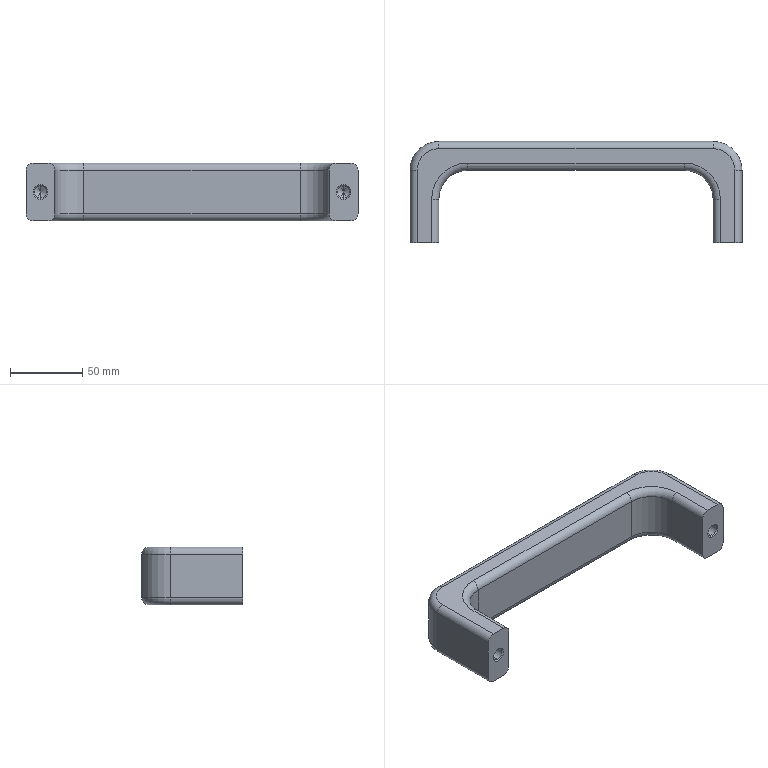Part | SolidWorks | features Fillet 2, 3DProfileFeature 1, Extrusion 1, HoleWzd 1 | 1 solid | 46 faces | box 230 x 70 x 40 mm | volume 254336 mm3 | cylinder 20 | plane 10 | cone 8 | torus 8 | commonest cylinder face diameters 10 x12 8.5 x4 40 x4
STEP:
#1=CARTESIAN_POINT('',(-31.,226.775,4.25));
#2=VERTEX_POINT('',#1);
#3=CARTESIAN_POINT('',(-31.,226.775,-4.25));
#4=VERTEX_POINT('',#3);
#5=CARTESIAN_POINT('',(-31.,226.775,0.));
#6=DIRECTION('',(0.,-1.,0.));
#7=DIRECTION('',(0.,0.,-1.));
#8=AXIS2_PLACEMENT_3D('',#5,#6,#7);
#9=CIRCLE('',#8,4.25);
#10=EDGE_CURVE('',#2,#4,#9,.T.);
#11=ORIENTED_EDGE('',*,*,#10,.F.);
#12=CARTESIAN_POINT('',(-31.,226.,5.025));
#13=VERTEX_POINT('',#12);
#14=CARTESIAN_POINT('',(-31.,226.,5.025));
#15=DIRECTION('',(0.,-0.7071,0.7071));
#16=VECTOR('',#15,1000.);
#17=LINE('',#14,#16);
#18=EDGE_CURVE('',#2,#13,#17,.T.);
#19=ORIENTED_EDGE('',*,*,#18,.T.);
#20=CARTESIAN_POINT('',(-31.,226.,-5.025));
#21=VERTEX_POINT('',#20);
#22=CARTESIAN_POINT('',(-31.,226.,0.));
#23=DIRECTION('',(0.,-1.,0.));
#24=DIRECTION('',(0.,0.,-1.));
#25=AXIS2_PLACEMENT_3D('',#22,#23,#24);
#26=CIRCLE('',#25,5.025);
#27=EDGE_CURVE('',#13,#21,#26,.T.);
#28=ORIENTED_EDGE('',*,*,#27,.T.);
#29=CARTESIAN_POINT('',(-31.,226.,-5.025));
#30=DIRECTION('',(0.,-0.7071,-0.7071));
#31=VECTOR('',#30,1000.);
#32=LINE('',#29,#31);
#33=EDGE_CURVE('',#4,#21,#32,.T.);
#34=ORIENTED_EDGE('',*,*,#33,.F.);
#35=EDGE_LOOP('',(#11,#19,#28,#34));
#36=FACE_OUTER_BOUND('',#35,.T.);
#37=CARTESIAN_POINT('',(-31.,226.,0.));
#38=DIRECTION('',(0.,-1.,0.));
#39=DIRECTION('',(0.,0.,-1.));
#40=AXIS2_PLACEMENT_3D('',#37,#38,#39);
#41=CONICAL_SURFACE('',#40,5.025,0.7854);
#42=ADVANCED_FACE('',(#36),#41,.F.);
#43=CARTESIAN_POINT('',(-31.,251.,4.25));
#44=VERTEX_POINT('',#43);
#45=CARTESIAN_POINT('',(-31.,251.,-4.25));
#46=VERTEX_POINT('',#45);
#47=CARTESIAN_POINT('',(-31.,251.,0.));
#48=DIRECTION('',(0.,-1.,0.));
#49=DIRECTION('',(0.,0.,-1.));
#50=AXIS2_PLACEMENT_3D('',#47,#48,#49);
#51=CIRCLE('',#50,4.25);
#52=EDGE_CURVE('',#44,#46,#51,.T.);
#53=ORIENTED_EDGE('',*,*,#52,.F.);
#54=CARTESIAN_POINT('',(-31.,226.,4.25));
#55=DIRECTION('',(0.,-1.,0.));
#56=VECTOR('',#55,1000.);
#57=LINE('',#54,#56);
#58=EDGE_CURVE('',#44,#2,#57,.T.);
#59=ORIENTED_EDGE('',*,*,#58,.T.);
#60=ORIENTED_EDGE('',*,*,#10,.T.);
#61=CARTESIAN_POINT('',(-31.,226.,-4.25));
#62=DIRECTION('',(0.,-1.,0.));
#63=VECTOR('',#62,1000.);
#64=LINE('',#61,#63);
#65=EDGE_CURVE('',#46,#4,#64,.T.);
#66=ORIENTED_EDGE('',*,*,#65,.F.);
#67=EDGE_LOOP('',(#53,#59,#60,#66));
#68=FACE_OUTER_BOUND('',#67,.T.);
#69=CARTESIAN_POINT('',(-31.,226.,0.));
#70=DIRECTION('',(0.,-1.,0.));
#71=DIRECTION('',(0.,0.,-1.));
#72=AXIS2_PLACEMENT_3D('',#69,#70,#71);
#73=CYLINDRICAL_SURFACE('',#72,4.25);
#74=ADVANCED_FACE('',(#68),#73,.F.);
#75=CARTESIAN_POINT('',(-31.,253.554,0.));
#76=VERTEX_POINT('',#75);
#77=CARTESIAN_POINT('',(-31.,251.,-4.25));
#78=DIRECTION('',(0.,-0.515,-0.8572));
#79=VECTOR('',#78,1000.);
#80=LINE('',#77,#79);
#81=EDGE_CURVE('',#76,#46,#80,.T.);
#82=ORIENTED_EDGE('',*,*,#81,.F.);
#83=CARTESIAN_POINT('',(-31.,251.,4.25));
#84=DIRECTION('',(0.,-0.515,0.8572));
#85=VECTOR('',#84,1000.);
#86=LINE('',#83,#85);
#87=EDGE_CURVE('',#76,#44,#86,.T.);
#88=ORIENTED_EDGE('',*,*,#87,.T.);
#89=ORIENTED_EDGE('',*,*,#52,.T.);
#90=EDGE_LOOP('',(#82,#88,#89));
#91=FACE_OUTER_BOUND('',#90,.T.);
#92=CARTESIAN_POINT('',(-31.,251.,0.));
#93=DIRECTION('',(0.,-1.,0.));
#94=DIRECTION('',(0.,0.,-1.));
#95=AXIS2_PLACEMENT_3D('',#92,#93,#94);
#96=CONICAL_SURFACE('',#95,4.25,1.03);
#97=ADVANCED_FACE('',(#91),#96,.F.);
#98=CARTESIAN_POINT('',(179.,226.775,4.25));
#99=VERTEX_POINT('',#98);
#100=CARTESIAN_POINT('',(179.,226.775,-4.25));
#101=VERTEX_POINT('',#100);
#102=CARTESIAN_POINT('',(179.,226.775,0.));
#103=DIRECTION('',(0.,-1.,0.));
#104=DIRECTION('',(0.,0.,-1.));
#105=AXIS2_PLACEMENT_3D('',#102,#103,#104);
#106=CIRCLE('',#105,4.25);
#107=EDGE_CURVE('',#99,#101,#106,.T.);
#108=ORIENTED_EDGE('',*,*,#107,.F.);
#109=CARTESIAN_POINT('',(179.,226.,5.025));
#110=VERTEX_POINT('',#109);
#111=CARTESIAN_POINT('',(179.,226.,5.025));
#112=DIRECTION('',(0.,-0.7071,0.7071));
#113=VECTOR('',#112,1000.);
#114=LINE('',#111,#113);
#115=EDGE_CURVE('',#99,#110,#114,.T.);
#116=ORIENTED_EDGE('',*,*,#115,.T.);
#117=CARTESIAN_POINT('',(179.,226.,-5.025));
#118=VERTEX_POINT('',#117);
#119=CARTESIAN_POINT('',(179.,226.,0.));
#120=DIRECTION('',(0.,-1.,0.));
#121=DIRECTION('',(0.,0.,-1.));
#122=AXIS2_PLACEMENT_3D('',#119,#120,#121);
#123=CIRCLE('',#122,5.025);
#124=EDGE_CURVE('',#110,#118,#123,.T.);
#125=ORIENTED_EDGE('',*,*,#124,.T.);
#126=CARTESIAN_POINT('',(179.,226.,-5.025));
#127=DIRECTION('',(0.,-0.7071,-0.7071));
#128=VECTOR('',#127,1000.);
#129=LINE('',#126,#128);
#130=EDGE_CURVE('',#101,#118,#129,.T.);
#131=ORIENTED_EDGE('',*,*,#130,.F.);
#132=EDGE_LOOP('',(#108,#116,#125,#131));
#133=FACE_OUTER_BOUND('',#132,.T.);
#134=CARTESIAN_POINT('',(179.,226.,0.));
#135=DIRECTION('',(0.,-1.,0.));
#136=DIRECTION('',(0.,0.,-1.));
#137=AXIS2_PLACEMENT_3D('',#134,#135,#136);
#138=CONICAL_SURFACE('',#137,5.025,0.7854);
#139=ADVANCED_FACE('',(#133),#138,.F.);
#140=CARTESIAN_POINT('',(179.,251.,4.25));
#141=VERTEX_POINT('',#140);
#142=CARTESIAN_POINT('',(179.,251.,-4.25));
#143=VERTEX_POINT('',#142);
#144=CARTESIAN_POINT('',(179.,251.,0.));
#145=DIRECTION('',(0.,-1.,0.));
#146=DIRECTION('',(0.,0.,-1.));
#147=AXIS2_PLACEMENT_3D('',#144,#145,#146);
#148=CIRCLE('',#147,4.25);
#149=EDGE_CURVE('',#141,#143,#148,.T.);
#150=ORIENTED_EDGE('',*,*,#149,.F.);
#151=CARTESIAN_POINT('',(179.,226.,4.25));
#152=DIRECTION('',(0.,-1.,0.));
#153=VECTOR('',#152,1000.);
#154=LINE('',#151,#153);
#155=EDGE_CURVE('',#141,#99,#154,.T.);
#156=ORIENTED_EDGE('',*,*,#155,.T.);
#157=ORIENTED_EDGE('',*,*,#107,.T.);
#158=CARTESIAN_POINT('',(179.,226.,-4.25));
#159=DIRECTION('',(0.,-1.,0.));
#160=VECTOR('',#159,1000.);
#161=LINE('',#158,#160);
#162=EDGE_CURVE('',#143,#101,#161,.T.);
#163=ORIENTED_EDGE('',*,*,#162,.F.);
#164=EDGE_LOOP('',(#150,#156,#157,#163));
#165=FACE_OUTER_BOUND('',#164,.T.);
#166=CARTESIAN_POINT('',(179.,226.,0.));
#167=DIRECTION('',(0.,-1.,0.));
#168=DIRECTION('',(0.,0.,-1.));
#169=AXIS2_PLACEMENT_3D('',#166,#167,#168);
#170=CYLINDRICAL_SURFACE('',#169,4.25);
#171=ADVANCED_FACE('',(#165),#170,.F.);
#172=CARTESIAN_POINT('',(179.,253.554,0.));
#173=VERTEX_POINT('',#172);
#174=CARTESIAN_POINT('',(179.,251.,-4.25));
#175=DIRECTION('',(0.,-0.515,-0.8572));
#176=VECTOR('',#175,1000.);
#177=LINE('',#174,#176);
#178=EDGE_CURVE('',#173,#143,#177,.T.);
#179=ORIENTED_EDGE('',*,*,#178,.F.);
#180=CARTESIAN_POINT('',(179.,251.,4.25));
#181=DIRECTION('',(0.,-0.515,0.8572));
#182=VECTOR('',#181,1000.);
#183=LINE('',#180,#182);
#184=EDGE_CURVE('',#173,#141,#183,.T.);
#185=ORIENTED_EDGE('',*,*,#184,.T.);
#186=ORIENTED_EDGE('',*,*,#149,.T.);
#187=EDGE_LOOP('',(#179,#185,#186));
#188=FACE_OUTER_BOUND('',#187,.T.);
#189=CARTESIAN_POINT('',(179.,251.,0.));
#190=DIRECTION('',(0.,-1.,0.));
#191=DIRECTION('',(0.,0.,-1.));
#192=AXIS2_PLACEMENT_3D('',#189,#190,#191);
#193=CONICAL_SURFACE('',#192,4.25,1.03);
#194=ADVANCED_FACE('',(#188),#193,.F.);
#195=CARTESIAN_POINT('',(-31.,226.,0.));
#196=DIRECTION('',(0.,-1.,0.));
#197=DIRECTION('',(0.,0.,-1.));
#198=AXIS2_PLACEMENT_3D('',#195,#196,#197);
#199=CIRCLE('',#198,5.025);
#200=EDGE_CURVE('',#21,#13,#199,.T.);
#201=ORIENTED_EDGE('',*,*,#200,.F.);
#202=ORIENTED_EDGE('',*,*,#27,.F.);
#203=EDGE_LOOP('',(#201,#202));
#204=FACE_BOUND('',#203,.T.);
#205=CARTESIAN_POINT('',(-41.,226.,15.));
#206=VERTEX_POINT('',#205);
#207=CARTESIAN_POINT('',(-41.,226.,-15.));
#208=VERTEX_POINT('',#207);
#209=CARTESIAN_POINT('',(-41.,226.,20.));
#210=DIRECTION('',(0.,0.,-1.));
#211=VECTOR('',#210,1000.);
#212=LINE('',#209,#211);
#213=EDGE_CURVE('',#206,#208,#212,.T.);
#214=ORIENTED_EDGE('',*,*,#213,.T.);
#215=CARTESIAN_POINT('',(-36.,226.,-20.));
#216=VERTEX_POINT('',#215);
#217=CARTESIAN_POINT('',(-36.,226.,-15.));
#218=DIRECTION('',(0.,-1.,0.));
#219=DIRECTION('',(0.,0.,-1.));
#220=AXIS2_PLACEMENT_3D('',#217,#218,#219);
#221=CIRCLE('',#220,5.);
#222=EDGE_CURVE('',#208,#216,#221,.T.);
#223=ORIENTED_EDGE('',*,*,#222,.T.);
#224=CARTESIAN_POINT('',(-26.,226.,-20.));
#225=VERTEX_POINT('',#224);
#226=CARTESIAN_POINT('',(-21.,226.,-20.));
#227=DIRECTION('',(-1.,0.,0.));
#228=VECTOR('',#227,1000.);
#229=LINE('',#226,#228);
#230=EDGE_CURVE('',#225,#216,#229,.T.);
#231=ORIENTED_EDGE('',*,*,#230,.F.);
#232=CARTESIAN_POINT('',(-21.,226.,-15.));
#233=VERTEX_POINT('',#232);
#234=CARTESIAN_POINT('',(-26.,226.,-15.));
#235=DIRECTION('',(0.,-1.,0.));
#236=DIRECTION('',(0.,0.,-1.));
#237=AXIS2_PLACEMENT_3D('',#234,#235,#236);
#238=CIRCLE('',#237,5.);
#239=EDGE_CURVE('',#225,#233,#238,.T.);
#240=ORIENTED_EDGE('',*,*,#239,.T.);
#241=CARTESIAN_POINT('',(-21.,226.,15.));
#242=VERTEX_POINT('',#241);
#243=CARTESIAN_POINT('',(-21.,226.,20.));
#244=DIRECTION('',(0.,0.,-1.));
#245=VECTOR('',#244,1000.);
#246=LINE('',#243,#245);
#247=EDGE_CURVE('',#242,#233,#246,.T.);
#248=ORIENTED_EDGE('',*,*,#247,.F.);
#249=CARTESIAN_POINT('',(-26.,226.,20.));
#250=VERTEX_POINT('',#249);
#251=CARTESIAN_POINT('',(-26.,226.,15.));
#252=DIRECTION('',(0.,-1.,0.));
#253=DIRECTION('',(0.,0.,-1.));
#254=AXIS2_PLACEMENT_3D('',#251,#252,#253);
#255=CIRCLE('',#254,5.);
#256=EDGE_CURVE('',#242,#250,#255,.T.);
#257=ORIENTED_EDGE('',*,*,#256,.T.);
#258=CARTESIAN_POINT('',(-36.,226.,20.));
#259=VERTEX_POINT('',#258);
#260=CARTESIAN_POINT('',(-21.,226.,20.));
#261=DIRECTION('',(-1.,0.,0.));
#262=VECTOR('',#261,1000.);
#263=LINE('',#260,#262);
#264=EDGE_CURVE('',#250,#259,#263,.T.);
#265=ORIENTED_EDGE('',*,*,#264,.T.);
#266=CARTESIAN_POINT('',(-36.,226.,15.));
#267=DIRECTION('',(0.,-1.,0.));
#268=DIRECTION('',(0.,0.,-1.));
#269=AXIS2_PLACEMENT_3D('',#266,#267,#268);
#270=CIRCLE('',#269,5.);
#271=EDGE_CURVE('',#259,#206,#270,.T.);
#272=ORIENTED_EDGE('',*,*,#271,.T.);
#273=EDGE_LOOP('',(#214,#223,#231,#240,#248,#257,#265,#272));
#274=FACE_OUTER_BOUND('',#273,.T.);
#275=CARTESIAN_POINT('',(-21.,226.,20.));
#276=DIRECTION('',(0.,-1.,0.));
#277=DIRECTION('',(0.,0.,-1.));
#278=AXIS2_PLACEMENT_3D('',#275,#276,#277);
#279=PLANE('',#278);
#280=ADVANCED_FACE('',(#204,#274),#279,.T.);
#281=ORIENTED_EDGE('',*,*,#247,.T.);
#282=CARTESIAN_POINT('',(-21.,256.,-15.));
#283=VERTEX_POINT('',#282);
#284=CARTESIAN_POINT('',(-21.,256.,-15.));
#285=DIRECTION('',(0.,1.,0.));
#286=VECTOR('',#285,1000.);
#287=LINE('',#284,#286);
#288=EDGE_CURVE('',#233,#283,#287,.T.);
#289=ORIENTED_EDGE('',*,*,#288,.T.);
#290=CARTESIAN_POINT('',(-21.,256.,15.));
#291=VERTEX_POINT('',#290);
#292=CARTESIAN_POINT('',(-21.,256.,20.));
#293=DIRECTION('',(0.,0.,1.));
#294=VECTOR('',#293,1000.);
#295=LINE('',#292,#294);
#296=EDGE_CURVE('',#283,#291,#295,.T.);
#297=ORIENTED_EDGE('',*,*,#296,.T.);
#298=CARTESIAN_POINT('',(-21.,226.,15.));
#299=DIRECTION('',(0.,-1.,0.));
#300=VECTOR('',#299,1000.);
#301=LINE('',#298,#300);
#302=EDGE_CURVE('',#291,#242,#301,.T.);
#303=ORIENTED_EDGE('',*,*,#302,.T.);
#304=EDGE_LOOP('',(#281,#289,#297,#303));
#305=FACE_OUTER_BOUND('',#304,.T.);
#306=CARTESIAN_POINT('',(-21.,226.,20.));
#307=DIRECTION('',(-1.,0.,0.));
#308=DIRECTION('',(0.,0.,1.));
#309=AXIS2_PLACEMENT_3D('',#306,#307,#308);
#310=PLANE('',#309);
#311=ADVANCED_FACE('',(#305),#310,.F.);
#312=CARTESIAN_POINT('',(-1.,276.,15.));
#313=VERTEX_POINT('',#312);
#314=CARTESIAN_POINT('',(-1.,276.,-15.));
#315=VERTEX_POINT('',#314);
#316=CARTESIAN_POINT('',(-1.,276.,-20.));
#317=DIRECTION('',(0.,0.,-1.));
#318=VECTOR('',#317,1000.);
#319=LINE('',#316,#318);
#320=EDGE_CURVE('',#313,#315,#319,.T.);
#321=ORIENTED_EDGE('',*,*,#320,.T.);
#322=CARTESIAN_POINT('',(149.,276.,-15.));
#323=VERTEX_POINT('',#322);
#324=CARTESIAN_POINT('',(149.,276.,-15.));
#325=DIRECTION('',(1.,0.,0.));
#326=VECTOR('',#325,1000.);
#327=LINE('',#324,#326);
#328=EDGE_CURVE('',#315,#323,#327,.T.);
#329=ORIENTED_EDGE('',*,*,#328,.T.);
#330=CARTESIAN_POINT('',(149.,276.,15.));
#331=VERTEX_POINT('',#330);
#332=CARTESIAN_POINT('',(149.,276.,20.));
#333=DIRECTION('',(0.,0.,1.));
#334=VECTOR('',#333,1000.);
#335=LINE('',#332,#334);
#336=EDGE_CURVE('',#323,#331,#335,.T.);
#337=ORIENTED_EDGE('',*,*,#336,.T.);
#338=CARTESIAN_POINT('',(-21.,276.,15.));
#339=DIRECTION('',(-1.,0.,0.));
#340=VECTOR('',#339,1000.);
#341=LINE('',#338,#340);
#342=EDGE_CURVE('',#331,#313,#341,.T.);
#343=ORIENTED_EDGE('',*,*,#342,.T.);
#344=EDGE_LOOP('',(#321,#329,#337,#343));
#345=FACE_OUTER_BOUND('',#344,.T.);
#346=CARTESIAN_POINT('',(-21.,276.,20.));
#347=DIRECTION('',(0.,1.,0.));
#348=DIRECTION('',(0.,0.,1.));
#349=AXIS2_PLACEMENT_3D('',#346,#347,#348);
#350=PLANE('',#349);
#351=ADVANCED_FACE('',(#345),#350,.F.);
#352=CARTESIAN_POINT('',(169.,256.,15.));
#353=VERTEX_POINT('',#352);
#354=CARTESIAN_POINT('',(169.,256.,-15.));
#355=VERTEX_POINT('',#354);
#356=CARTESIAN_POINT('',(169.,256.,-20.));
#357=DIRECTION('',(0.,0.,-1.));
#358=VECTOR('',#357,1000.);
#359=LINE('',#356,#358);
#360=EDGE_CURVE('',#353,#355,#359,.T.);
#361=ORIENTED_EDGE('',*,*,#360,.T.);
#362=CARTESIAN_POINT('',(169.,226.,-15.));
#363=VERTEX_POINT('',#362);
#364=CARTESIAN_POINT('',(169.,226.,-15.));
#365=DIRECTION('',(0.,-1.,0.));
#366=VECTOR('',#365,1000.);
#367=LINE('',#364,#366);
#368=EDGE_CURVE('',#355,#363,#367,.T.);
#369=ORIENTED_EDGE('',*,*,#368,.T.);
#370=CARTESIAN_POINT('',(169.,226.,15.));
#371=VERTEX_POINT('',#370);
#372=CARTESIAN_POINT('',(169.,226.,20.));
#373=DIRECTION('',(0.,0.,-1.));
#374=VECTOR('',#373,1000.);
#375=LINE('',#372,#374);
#376=EDGE_CURVE('',#371,#363,#375,.T.);
#377=ORIENTED_EDGE('',*,*,#376,.F.);
#378=CARTESIAN_POINT('',(169.,276.,15.));
#379=DIRECTION('',(0.,1.,0.));
#380=VECTOR('',#379,1000.);
#381=LINE('',#378,#380);
#382=EDGE_CURVE('',#371,#353,#381,.T.);
#383=ORIENTED_EDGE('',*,*,#382,.T.);
#384=EDGE_LOOP('',(#361,#369,#377,#383));
#385=FACE_OUTER_BOUND('',#384,.T.);
#386=CARTESIAN_POINT('',(169.,276.,20.));
#387=DIRECTION('',(1.,0.,0.));
#388=DIRECTION('',(0.,0.,-1.));
#389=AXIS2_PLACEMENT_3D('',#386,#387,#388);
#390=PLANE('',#389);
#391=ADVANCED_FACE('',(#385),#390,.F.);
#392=CARTESIAN_POINT('',(179.,226.,0.));
#393=DIRECTION('',(0.,-1.,0.));
#394=DIRECTION('',(0.,0.,-1.));
#395=AXIS2_PLACEMENT_3D('',#392,#393,#394);
#396=CIRCLE('',#395,5.025);
#397=EDGE_CURVE('',#118,#110,#396,.T.);
#398=ORIENTED_EDGE('',*,*,#397,.F.);
#399=ORIENTED_EDGE('',*,*,#124,.F.);
#400=EDGE_LOOP('',(#398,#399));
#401=FACE_BOUND('',#400,.T.);
#402=ORIENTED_EDGE('',*,*,#376,.T.);
#403=CARTESIAN_POINT('',(174.,226.,-20.));
#404=VERTEX_POINT('',#403);
#405=CARTESIAN_POINT('',(174.,226.,-15.));
#406=DIRECTION('',(0.,-1.,0.));
#407=DIRECTION('',(0.,0.,-1.));
#408=AXIS2_PLACEMENT_3D('',#405,#406,#407);
#409=CIRCLE('',#408,5.);
#410=EDGE_CURVE('',#363,#404,#409,.T.);
#411=ORIENTED_EDGE('',*,*,#410,.T.);
#412=CARTESIAN_POINT('',(184.,226.,-20.));
#413=VERTEX_POINT('',#412);
#414=CARTESIAN_POINT('',(189.,226.,-20.));
#415=DIRECTION('',(-1.,0.,0.));
#416=VECTOR('',#415,1000.);
#417=LINE('',#414,#416);
#418=EDGE_CURVE('',#413,#404,#417,.T.);
#419=ORIENTED_EDGE('',*,*,#418,.F.);
#420=CARTESIAN_POINT('',(189.,226.,-15.));
#421=VERTEX_POINT('',#420);
#422=CARTESIAN_POINT('',(184.,226.,-15.));
#423=DIRECTION('',(0.,-1.,0.));
#424=DIRECTION('',(0.,0.,-1.));
#425=AXIS2_PLACEMENT_3D('',#422,#423,#424);
#426=CIRCLE('',#425,5.);
#427=EDGE_CURVE('',#413,#421,#426,.T.);
#428=ORIENTED_EDGE('',*,*,#427,.T.);
#429=CARTESIAN_POINT('',(189.,226.,15.));
#430=VERTEX_POINT('',#429);
#431=CARTESIAN_POINT('',(189.,226.,20.));
#432=DIRECTION('',(0.,0.,-1.));
#433=VECTOR('',#432,1000.);
#434=LINE('',#431,#433);
#435=EDGE_CURVE('',#430,#421,#434,.T.);
#436=ORIENTED_EDGE('',*,*,#435,.F.);
#437=CARTESIAN_POINT('',(184.,226.,20.));
#438=VERTEX_POINT('',#437);
#439=CARTESIAN_POINT('',(184.,226.,15.));
#440=DIRECTION('',(0.,-1.,0.));
#441=DIRECTION('',(0.,0.,-1.));
#442=AXIS2_PLACEMENT_3D('',#439,#440,#441);
#443=CIRCLE('',#442,5.);
#444=EDGE_CURVE('',#430,#438,#443,.T.);
#445=ORIENTED_EDGE('',*,*,#444,.T.);
#446=CARTESIAN_POINT('',(174.,226.,20.));
#447=VERTEX_POINT('',#446);
#448=CARTESIAN_POINT('',(189.,226.,20.));
#449=DIRECTION('',(-1.,0.,0.));
#450=VECTOR('',#449,1000.);
#451=LINE('',#448,#450);
#452=EDGE_CURVE('',#438,#447,#451,.T.);
#453=ORIENTED_EDGE('',*,*,#452,.T.);
#454=CARTESIAN_POINT('',(174.,226.,15.));
#455=DIRECTION('',(0.,-1.,0.));
#456=DIRECTION('',(0.,0.,-1.));
#457=AXIS2_PLACEMENT_3D('',#454,#455,#456);
#458=CIRCLE('',#457,5.);
#459=EDGE_CURVE('',#447,#371,#458,.T.);
#460=ORIENTED_EDGE('',*,*,#459,.T.);
#461=EDGE_LOOP('',(#402,#411,#419,#428,#436,#445,#453,#460));
#462=FACE_OUTER_BOUND('',#461,.T.);
#463=CARTESIAN_POINT('',(189.,226.,20.));
#464=DIRECTION('',(0.,-1.,0.));
#465=DIRECTION('',(0.,0.,-1.));
#466=AXIS2_PLACEMENT_3D('',#463,#464,#465);
#467=PLANE('',#466);
#468=ADVANCED_FACE('',(#401,#462),#467,.T.);
#469=ORIENTED_EDGE('',*,*,#435,.T.);
#470=CARTESIAN_POINT('',(189.,276.,-15.));
#471=VERTEX_POINT('',#470);
#472=CARTESIAN_POINT('',(189.,296.,-15.));
#473=DIRECTION('',(0.,1.,0.));
#474=VECTOR('',#473,1000.);
#475=LINE('',#472,#474);
#476=EDGE_CURVE('',#421,#471,#475,.T.);
#477=ORIENTED_EDGE('',*,*,#476,.T.);
#478=CARTESIAN_POINT('',(189.,276.,15.));
#479=VERTEX_POINT('',#478);
#480=CARTESIAN_POINT('',(189.,276.,20.));
#481=DIRECTION('',(0.,0.,1.));
#482=VECTOR('',#481,1000.);
#483=LINE('',#480,#482);
#484=EDGE_CURVE('',#471,#479,#483,.T.);
#485=ORIENTED_EDGE('',*,*,#484,.T.);
#486=CARTESIAN_POINT('',(189.,226.,15.));
#487=DIRECTION('',(0.,-1.,0.));
#488=VECTOR('',#487,1000.);
#489=LINE('',#486,#488);
#490=EDGE_CURVE('',#479,#430,#489,.T.);
#491=ORIENTED_EDGE('',*,*,#490,.T.);
#492=EDGE_LOOP('',(#469,#477,#485,#491));
#493=FACE_OUTER_BOUND('',#492,.T.);
#494=CARTESIAN_POINT('',(189.,296.,20.));
#495=DIRECTION('',(1.,0.,0.));
#496=DIRECTION('',(0.,0.,-1.));
#497=AXIS2_PLACEMENT_3D('',#494,#495,#496);
#498=PLANE('',#497);
#499=ADVANCED_FACE('',(#493),#498,.T.);
#500=CARTESIAN_POINT('',(169.,296.,15.));
#501=VERTEX_POINT('',#500);
#502=CARTESIAN_POINT('',(169.,296.,-15.));
#503=VERTEX_POINT('',#502);
#504=CARTESIAN_POINT('',(169.,296.,20.));
#505=DIRECTION('',(0.,0.,-1.));
#506=VECTOR('',#505,1000.);
#507=LINE('',#504,#506);
#508=EDGE_CURVE('',#501,#503,#507,.T.);
#509=ORIENTED_EDGE('',*,*,#508,.T.);
#510=CARTESIAN_POINT('',(-21.,296.,-15.));
#511=VERTEX_POINT('',#510);
#512=CARTESIAN_POINT('',(-41.,296.,-15.));
#513=DIRECTION('',(-1.,0.,0.));
#514=VECTOR('',#513,1000.);
#515=LINE('',#512,#514);
#516=EDGE_CURVE('',#503,#511,#515,.T.);
#517=ORIENTED_EDGE('',*,*,#516,.T.);
#518=CARTESIAN_POINT('',(-21.,296.,15.));
#519=VERTEX_POINT('',#518);
#520=CARTESIAN_POINT('',(-21.,296.,20.));
#521=DIRECTION('',(0.,0.,1.));
#522=VECTOR('',#521,1000.);
#523=LINE('',#520,#522);
#524=EDGE_CURVE('',#511,#519,#523,.T.);
#525=ORIENTED_EDGE('',*,*,#524,.T.);
#526=CARTESIAN_POINT('',(169.,296.,15.));
#527=DIRECTION('',(1.,0.,0.));
#528=VECTOR('',#527,1000.);
#529=LINE('',#526,#528);
#530=EDGE_CURVE('',#519,#501,#529,.T.);
#531=ORIENTED_EDGE('',*,*,#530,.T.);
#532=EDGE_LOOP('',(#509,#517,#525,#531));
#533=FACE_OUTER_BOUND('',#532,.T.);
#534=CARTESIAN_POINT('',(-41.,296.,20.));
#535=DIRECTION('',(0.,1.,0.));
#536=DIRECTION('',(0.,0.,1.));
#537=AXIS2_PLACEMENT_3D('',#534,#535,#536);
#538=PLANE('',#537);
#539=ADVANCED_FACE('',(#533),#538,.T.);
#540=CARTESIAN_POINT('',(-41.,276.,15.));
#541=VERTEX_POINT('',#540);
#542=CARTESIAN_POINT('',(-41.,276.,-15.));
#543=VERTEX_POINT('',#542);
#544=CARTESIAN_POINT('',(-41.,276.,20.));
#545=DIRECTION('',(0.,0.,-1.));
#546=VECTOR('',#545,1000.);
#547=LINE('',#544,#546);
#548=EDGE_CURVE('',#541,#543,#547,.T.);
#549=ORIENTED_EDGE('',*,*,#548,.T.);
#550=CARTESIAN_POINT('',(-41.,226.,-15.));
#551=DIRECTION('',(0.,-1.,0.));
#552=VECTOR('',#551,1000.);
#553=LINE('',#550,#552);
#554=EDGE_CURVE('',#543,#208,#553,.T.);
#555=ORIENTED_EDGE('',*,*,#554,.T.);
#556=ORIENTED_EDGE('',*,*,#213,.F.);
#557=CARTESIAN_POINT('',(-41.,276.,15.));
#558=DIRECTION('',(0.,1.,0.));
#559=VECTOR('',#558,1000.);
#560=LINE('',#557,#559);
#561=EDGE_CURVE('',#206,#541,#560,.T.);
#562=ORIENTED_EDGE('',*,*,#561,.T.);
#563=EDGE_LOOP('',(#549,#555,#556,#562));
#564=FACE_OUTER_BOUND('',#563,.T.);
#565=CARTESIAN_POINT('',(-41.,226.,20.));
#566=DIRECTION('',(-1.,0.,0.));
#567=DIRECTION('',(0.,-1.,0.));
#568=AXIS2_PLACEMENT_3D('',#565,#566,#567);
#569=PLANE('',#568);
#570=ADVANCED_FACE('',(#564),#569,.T.);
#571=CARTESIAN_POINT('',(149.,281.,20.));
#572=VERTEX_POINT('',#571);
#573=CARTESIAN_POINT('',(174.,256.,20.));
#574=VERTEX_POINT('',#573);
#575=CARTESIAN_POINT('',(149.,256.,20.));
#576=DIRECTION('',(0.,0.,-1.));
#577=DIRECTION('',(-1.,0.,0.));
#578=AXIS2_PLACEMENT_3D('',#575,#576,#577);
#579=CIRCLE('',#578,25.);
#580=EDGE_CURVE('',#572,#574,#579,.T.);
#581=ORIENTED_EDGE('',*,*,#580,.T.);
#582=CARTESIAN_POINT('',(174.,0.,20.));
#583=DIRECTION('',(0.,-1.,0.));
#584=VECTOR('',#583,1000.);
#585=LINE('',#582,#584);
#586=EDGE_CURVE('',#574,#447,#585,.T.);
#587=ORIENTED_EDGE('',*,*,#586,.T.);
#588=ORIENTED_EDGE('',*,*,#452,.F.);
#589=CARTESIAN_POINT('',(184.,276.,20.));
#590=VERTEX_POINT('',#589);
#591=CARTESIAN_POINT('',(184.,276.,20.));
#592=DIRECTION('',(0.,1.,0.));
#593=VECTOR('',#592,1000.);
#594=LINE('',#591,#593);
#595=EDGE_CURVE('',#438,#590,#594,.T.);
#596=ORIENTED_EDGE('',*,*,#595,.T.);
#597=CARTESIAN_POINT('',(169.,291.,20.));
#598=VERTEX_POINT('',#597);
#599=CARTESIAN_POINT('',(169.,276.,20.));
#600=DIRECTION('',(0.,0.,1.));
#601=DIRECTION('',(-1.,0.,0.));
#602=AXIS2_PLACEMENT_3D('',#599,#600,#601);
#603=CIRCLE('',#602,15.);
#604=EDGE_CURVE('',#590,#598,#603,.T.);
#605=ORIENTED_EDGE('',*,*,#604,.T.);
#606=CARTESIAN_POINT('',(-21.,291.,20.));
#607=VERTEX_POINT('',#606);
#608=CARTESIAN_POINT('',(-21.,291.,20.));
#609=DIRECTION('',(-1.,0.,0.));
#610=VECTOR('',#609,1000.);
#611=LINE('',#608,#610);
#612=EDGE_CURVE('',#598,#607,#611,.T.);
#613=ORIENTED_EDGE('',*,*,#612,.T.);
#614=CARTESIAN_POINT('',(-36.,276.,20.));
#615=VERTEX_POINT('',#614);
#616=CARTESIAN_POINT('',(-21.,276.,20.));
#617=DIRECTION('',(0.,0.,1.));
#618=DIRECTION('',(-1.,0.,0.));
#619=AXIS2_PLACEMENT_3D('',#616,#617,#618);
#620=CIRCLE('',#619,15.);
#621=EDGE_CURVE('',#607,#615,#620,.T.);
#622=ORIENTED_EDGE('',*,*,#621,.T.);
#623=CARTESIAN_POINT('',(-36.,226.,20.));
#624=DIRECTION('',(0.,-1.,0.));
#625=VECTOR('',#624,1000.);
#626=LINE('',#623,#625);
#627=EDGE_CURVE('',#615,#259,#626,.T.);
#628=ORIENTED_EDGE('',*,*,#627,.T.);
#629=ORIENTED_EDGE('',*,*,#264,.F.);
#630=CARTESIAN_POINT('',(-26.,256.,20.));
#631=VERTEX_POINT('',#630);
#632=CARTESIAN_POINT('',(-26.,0.,20.));
#633=DIRECTION('',(0.,1.,0.));
#634=VECTOR('',#633,1000.);
#635=LINE('',#632,#634);
#636=EDGE_CURVE('',#250,#631,#635,.T.);
#637=ORIENTED_EDGE('',*,*,#636,.T.);
#638=CARTESIAN_POINT('',(-1.,281.,20.));
#639=VERTEX_POINT('',#638);
#640=CARTESIAN_POINT('',(-1.,256.,20.));
#641=DIRECTION('',(0.,0.,-1.));
#642=DIRECTION('',(-1.,0.,0.));
#643=AXIS2_PLACEMENT_3D('',#640,#641,#642);
#644=CIRCLE('',#643,25.);
#645=EDGE_CURVE('',#631,#639,#644,.T.);
#646=ORIENTED_EDGE('',*,*,#645,.T.);
#647=CARTESIAN_POINT('',(0.,281.,20.));
#648=DIRECTION('',(1.,0.,0.));
#649=VECTOR('',#648,1000.);
#650=LINE('',#647,#649);
#651=EDGE_CURVE('',#639,#572,#650,.T.);
#652=ORIENTED_EDGE('',*,*,#651,.T.);
#653=EDGE_LOOP('',(#581,#587,#588,#596,#605,#613,#622,#628,#629,#637,#646,#652));
#654=FACE_OUTER_BOUND('',#653,.T.);
#655=CARTESIAN_POINT('',(0.,0.,20.));
#656=DIRECTION('',(0.,0.,-1.));
#657=DIRECTION('',(-1.,0.,0.));
#658=AXIS2_PLACEMENT_3D('',#655,#656,#657);
#659=PLANE('',#658);
#660=ADVANCED_FACE('',(#654),#659,.F.);
#661=ORIENTED_EDGE('',*,*,#418,.T.);
#662=CARTESIAN_POINT('',(174.,256.,-20.));
#663=VERTEX_POINT('',#662);
#664=CARTESIAN_POINT('',(174.,256.,-20.));
#665=DIRECTION('',(0.,1.,0.));
#666=VECTOR('',#665,1000.);
#667=LINE('',#664,#666);
#668=EDGE_CURVE('',#404,#663,#667,.T.);
#669=ORIENTED_EDGE('',*,*,#668,.T.);
#670=CARTESIAN_POINT('',(149.,281.,-20.));
#671=VERTEX_POINT('',#670);
#672=CARTESIAN_POINT('',(149.,256.,-20.));
#673=DIRECTION('',(0.,0.,1.));
#674=DIRECTION('',(-1.,0.,0.));
#675=AXIS2_PLACEMENT_3D('',#672,#673,#674);
#676=CIRCLE('',#675,25.);
#677=EDGE_CURVE('',#663,#671,#676,.T.);
#678=ORIENTED_EDGE('',*,*,#677,.T.);
#679=CARTESIAN_POINT('',(-1.,281.,-20.));
#680=VERTEX_POINT('',#679);
#681=CARTESIAN_POINT('',(-1.,281.,-20.));
#682=DIRECTION('',(-1.,0.,0.));
#683=VECTOR('',#682,1000.);
#684=LINE('',#681,#683);
#685=EDGE_CURVE('',#671,#680,#684,.T.);
#686=ORIENTED_EDGE('',*,*,#685,.T.);
#687=CARTESIAN_POINT('',(-26.,256.,-20.));
#688=VERTEX_POINT('',#687);
#689=CARTESIAN_POINT('',(-1.,256.,-20.));
#690=DIRECTION('',(0.,0.,1.));
#691=DIRECTION('',(-1.,0.,0.));
#692=AXIS2_PLACEMENT_3D('',#689,#690,#691);
#693=CIRCLE('',#692,25.);
#694=EDGE_CURVE('',#680,#688,#693,.T.);
#695=ORIENTED_EDGE('',*,*,#694,.T.);
#696=CARTESIAN_POINT('',(-26.,226.,-20.));
#697=DIRECTION('',(0.,-1.,0.));
#698=VECTOR('',#697,1000.);
#699=LINE('',#696,#698);
#700=EDGE_CURVE('',#688,#225,#699,.T.);
#701=ORIENTED_EDGE('',*,*,#700,.T.);
#702=ORIENTED_EDGE('',*,*,#230,.T.);
#703=CARTESIAN_POINT('',(-36.,276.,-20.));
#704=VERTEX_POINT('',#703);
#705=CARTESIAN_POINT('',(-36.,0.,-20.));
#706=DIRECTION('',(0.,1.,0.));
#707=VECTOR('',#706,1000.);
#708=LINE('',#705,#707);
#709=EDGE_CURVE('',#216,#704,#708,.T.);
#710=ORIENTED_EDGE('',*,*,#709,.T.);
#711=CARTESIAN_POINT('',(-21.,291.,-20.));
#712=VERTEX_POINT('',#711);
#713=CARTESIAN_POINT('',(-21.,276.,-20.));
#714=DIRECTION('',(0.,0.,-1.));
#715=DIRECTION('',(-1.,0.,0.));
#716=AXIS2_PLACEMENT_3D('',#713,#714,#715);
#717=CIRCLE('',#716,15.);
#718=EDGE_CURVE('',#704,#712,#717,.T.);
#719=ORIENTED_EDGE('',*,*,#718,.T.);
#720=CARTESIAN_POINT('',(169.,291.,-20.));
#721=VERTEX_POINT('',#720);
#722=CARTESIAN_POINT('',(0.,291.,-20.));
#723=DIRECTION('',(1.,0.,0.));
#724=VECTOR('',#723,1000.);
#725=LINE('',#722,#724);
#726=EDGE_CURVE('',#712,#721,#725,.T.);
#727=ORIENTED_EDGE('',*,*,#726,.T.);
#728=CARTESIAN_POINT('',(184.,276.,-20.));
#729=VERTEX_POINT('',#728);
#730=CARTESIAN_POINT('',(169.,276.,-20.));
#731=DIRECTION('',(0.,0.,-1.));
#732=DIRECTION('',(-1.,0.,0.));
#733=AXIS2_PLACEMENT_3D('',#730,#731,#732);
#734=CIRCLE('',#733,15.);
#735=EDGE_CURVE('',#721,#729,#734,.T.);
#736=ORIENTED_EDGE('',*,*,#735,.T.);
#737=CARTESIAN_POINT('',(184.,0.,-20.));
#738=DIRECTION('',(0.,-1.,0.));
#739=VECTOR('',#738,1000.);
#740=LINE('',#737,#739);
#741=EDGE_CURVE('',#729,#413,#740,.T.);
#742=ORIENTED_EDGE('',*,*,#741,.T.);
#743=EDGE_LOOP('',(#661,#669,#678,#686,#695,#701,#702,#710,#719,#727,#736,#742));
#744=FACE_OUTER_BOUND('',#743,.T.);
#745=CARTESIAN_POINT('',(0.,0.,-20.));
#746=DIRECTION('',(0.,0.,-1.));
#747=DIRECTION('',(-1.,0.,0.));
#748=AXIS2_PLACEMENT_3D('',#745,#746,#747);
#749=PLANE('',#748);
#750=ADVANCED_FACE('',(#744),#749,.T.);
#751=ORIENTED_EDGE('',*,*,#484,.F.);
#752=CARTESIAN_POINT('',(169.,276.,-15.));
#753=DIRECTION('',(0.,0.,1.));
#754=DIRECTION('',(-1.,0.,0.));
#755=AXIS2_PLACEMENT_3D('',#752,#753,#754);
#756=CIRCLE('',#755,20.);
#757=EDGE_CURVE('',#471,#503,#756,.T.);
#758=ORIENTED_EDGE('',*,*,#757,.T.);
#759=ORIENTED_EDGE('',*,*,#508,.F.);
#760=CARTESIAN_POINT('',(169.,276.,15.));
#761=DIRECTION('',(0.,0.,-1.));
#762=DIRECTION('',(-1.,0.,0.));
#763=AXIS2_PLACEMENT_3D('',#760,#761,#762);
#764=CIRCLE('',#763,20.);
#765=EDGE_CURVE('',#501,#479,#764,.T.);
#766=ORIENTED_EDGE('',*,*,#765,.T.);
#767=EDGE_LOOP('',(#751,#758,#759,#766));
#768=FACE_OUTER_BOUND('',#767,.T.);
#769=CARTESIAN_POINT('',(169.,276.,20.));
#770=DIRECTION('',(0.,0.,-1.));
#771=DIRECTION('',(-1.,0.,0.));
#772=AXIS2_PLACEMENT_3D('',#769,#770,#771);
#773=CYLINDRICAL_SURFACE('',#772,20.);
#774=ADVANCED_FACE('',(#768),#773,.T.);
#775=ORIENTED_EDGE('',*,*,#336,.F.);
#776=CARTESIAN_POINT('',(149.,256.,-15.));
#777=DIRECTION('',(0.,0.,-1.));
#778=DIRECTION('',(-1.,0.,0.));
#779=AXIS2_PLACEMENT_3D('',#776,#777,#778);
#780=CIRCLE('',#779,20.);
#781=EDGE_CURVE('',#323,#355,#780,.T.);
#782=ORIENTED_EDGE('',*,*,#781,.T.);
#783=ORIENTED_EDGE('',*,*,#360,.F.);
#784=CARTESIAN_POINT('',(149.,256.,15.));
#785=DIRECTION('',(0.,0.,1.));
#786=DIRECTION('',(-1.,0.,0.));
#787=AXIS2_PLACEMENT_3D('',#784,#785,#786);
#788=CIRCLE('',#787,20.);
#789=EDGE_CURVE('',#353,#331,#788,.T.);
#790=ORIENTED_EDGE('',*,*,#789,.T.);
#791=EDGE_LOOP('',(#775,#782,#783,#790));
#792=FACE_OUTER_BOUND('',#791,.T.);
#793=CARTESIAN_POINT('',(149.,256.,20.));
#794=DIRECTION('',(0.,0.,1.));
#795=DIRECTION('',(1.,0.,0.));
#796=AXIS2_PLACEMENT_3D('',#793,#794,#795);
#797=CYLINDRICAL_SURFACE('',#796,20.);
#798=ADVANCED_FACE('',(#792),#797,.F.);
#799=ORIENTED_EDGE('',*,*,#296,.F.);
#800=CARTESIAN_POINT('',(-1.,256.,-15.));
#801=DIRECTION('',(0.,0.,-1.));
#802=DIRECTION('',(-1.,0.,0.));
#803=AXIS2_PLACEMENT_3D('',#800,#801,#802);
#804=CIRCLE('',#803,20.);
#805=EDGE_CURVE('',#283,#315,#804,.T.);
#806=ORIENTED_EDGE('',*,*,#805,.T.);
#807=ORIENTED_EDGE('',*,*,#320,.F.);
#808=CARTESIAN_POINT('',(-1.,256.,15.));
#809=DIRECTION('',(0.,0.,1.));
#810=DIRECTION('',(-1.,0.,0.));
#811=AXIS2_PLACEMENT_3D('',#808,#809,#810);
#812=CIRCLE('',#811,20.);
#813=EDGE_CURVE('',#313,#291,#812,.T.);
#814=ORIENTED_EDGE('',*,*,#813,.T.);
#815=EDGE_LOOP('',(#799,#806,#807,#814));
#816=FACE_OUTER_BOUND('',#815,.T.);
#817=CARTESIAN_POINT('',(-1.,256.,20.));
#818=DIRECTION('',(0.,0.,1.));
#819=DIRECTION('',(1.,0.,0.));
#820=AXIS2_PLACEMENT_3D('',#817,#818,#819);
#821=CYLINDRICAL_SURFACE('',#820,20.);
#822=ADVANCED_FACE('',(#816),#821,.F.);
#823=ORIENTED_EDGE('',*,*,#524,.F.);
#824=CARTESIAN_POINT('',(-21.,276.,-15.));
#825=DIRECTION('',(0.,0.,1.));
#826=DIRECTION('',(-1.,0.,0.));
#827=AXIS2_PLACEMENT_3D('',#824,#825,#826);
#828=CIRCLE('',#827,20.);
#829=EDGE_CURVE('',#511,#543,#828,.T.);
#830=ORIENTED_EDGE('',*,*,#829,.T.);
#831=ORIENTED_EDGE('',*,*,#548,.F.);
#832=CARTESIAN_POINT('',(-21.,276.,15.));
#833=DIRECTION('',(0.,0.,-1.));
#834=DIRECTION('',(-1.,0.,0.));
#835=AXIS2_PLACEMENT_3D('',#832,#833,#834);
#836=CIRCLE('',#835,20.);
#837=EDGE_CURVE('',#541,#519,#836,.T.);
#838=ORIENTED_EDGE('',*,*,#837,.T.);
#839=EDGE_LOOP('',(#823,#830,#831,#838));
#840=FACE_OUTER_BOUND('',#839,.T.);
#841=CARTESIAN_POINT('',(-21.,276.,20.));
#842=DIRECTION('',(0.,0.,-1.));
#843=DIRECTION('',(-1.,0.,0.));
#844=AXIS2_PLACEMENT_3D('',#841,#842,#843);
#845=CYLINDRICAL_SURFACE('',#844,20.);
#846=ADVANCED_FACE('',(#840),#845,.T.);
#847=ORIENTED_EDGE('',*,*,#239,.F.);
#848=ORIENTED_EDGE('',*,*,#700,.F.);
#849=CARTESIAN_POINT('',(-26.,256.,-15.));
#850=DIRECTION('',(0.,1.,0.));
#851=DIRECTION('',(0.,0.,1.));
#852=AXIS2_PLACEMENT_3D('',#849,#850,#851);
#853=CIRCLE('',#852,5.);
#854=EDGE_CURVE('',#283,#688,#853,.T.);
#855=ORIENTED_EDGE('',*,*,#854,.F.);
#856=ORIENTED_EDGE('',*,*,#288,.F.);
#857=EDGE_LOOP('',(#847,#848,#855,#856));
#858=FACE_OUTER_BOUND('',#857,.T.);
#859=CARTESIAN_POINT('',(-26.,226.,-15.));
#860=DIRECTION('',(0.,-1.,0.));
#861=DIRECTION('',(0.,0.,-1.));
#862=AXIS2_PLACEMENT_3D('',#859,#860,#861);
#863=CYLINDRICAL_SURFACE('',#862,5.);
#864=ADVANCED_FACE('',(#858),#863,.T.);
#865=ORIENTED_EDGE('',*,*,#854,.T.);
#866=ORIENTED_EDGE('',*,*,#694,.F.);
#867=CARTESIAN_POINT('',(-1.,281.,-15.));
#868=DIRECTION('',(1.,0.,0.));
#869=DIRECTION('',(0.,0.,-1.));
#870=AXIS2_PLACEMENT_3D('',#867,#868,#869);
#871=CIRCLE('',#870,5.);
#872=EDGE_CURVE('',#315,#680,#871,.T.);
#873=ORIENTED_EDGE('',*,*,#872,.F.);
#874=ORIENTED_EDGE('',*,*,#805,.F.);
#875=EDGE_LOOP('',(#865,#866,#873,#874));
#876=FACE_OUTER_BOUND('',#875,.T.);
#877=CARTESIAN_POINT('',(-1.,256.,-15.));
#878=DIRECTION('',(0.,0.,-1.));
#879=DIRECTION('',(-1.,0.,0.));
#880=AXIS2_PLACEMENT_3D('',#877,#878,#879);
#881=TOROIDAL_SURFACE('',#880,25.,5.);
#882=ADVANCED_FACE('',(#876),#881,.T.);
#883=ORIENTED_EDGE('',*,*,#872,.T.);
#884=ORIENTED_EDGE('',*,*,#685,.F.);
#885=CARTESIAN_POINT('',(149.,281.,-15.));
#886=DIRECTION('',(1.,0.,0.));
#887=DIRECTION('',(0.,0.,-1.));
#888=AXIS2_PLACEMENT_3D('',#885,#886,#887);
#889=CIRCLE('',#888,5.);
#890=EDGE_CURVE('',#323,#671,#889,.T.);
#891=ORIENTED_EDGE('',*,*,#890,.F.);
#892=ORIENTED_EDGE('',*,*,#328,.F.);
#893=EDGE_LOOP('',(#883,#884,#891,#892));
#894=FACE_OUTER_BOUND('',#893,.T.);
#895=CARTESIAN_POINT('',(-21.,281.,-15.));
#896=DIRECTION('',(-1.,0.,0.));
#897=DIRECTION('',(0.,0.,1.));
#898=AXIS2_PLACEMENT_3D('',#895,#896,#897);
#899=CYLINDRICAL_SURFACE('',#898,5.);
#900=ADVANCED_FACE('',(#894),#899,.T.);
#901=ORIENTED_EDGE('',*,*,#890,.T.);
#902=ORIENTED_EDGE('',*,*,#677,.F.);
#903=CARTESIAN_POINT('',(174.,256.,-15.));
#904=DIRECTION('',(0.,-1.,0.));
#905=DIRECTION('',(0.,0.,-1.));
#906=AXIS2_PLACEMENT_3D('',#903,#904,#905);
#907=CIRCLE('',#906,5.);
#908=EDGE_CURVE('',#355,#663,#907,.T.);
#909=ORIENTED_EDGE('',*,*,#908,.F.);
#910=ORIENTED_EDGE('',*,*,#781,.F.);
#911=EDGE_LOOP('',(#901,#902,#909,#910));
#912=FACE_OUTER_BOUND('',#911,.T.);
#913=CARTESIAN_POINT('',(149.,256.,-15.));
#914=DIRECTION('',(0.,0.,-1.));
#915=DIRECTION('',(-1.,0.,0.));
#916=AXIS2_PLACEMENT_3D('',#913,#914,#915);
#917=TOROIDAL_SURFACE('',#916,25.,5.);
#918=ADVANCED_FACE('',(#912),#917,.T.);
#919=ORIENTED_EDGE('',*,*,#908,.T.);
#920=ORIENTED_EDGE('',*,*,#668,.F.);
#921=ORIENTED_EDGE('',*,*,#410,.F.);
#922=ORIENTED_EDGE('',*,*,#368,.F.);
#923=EDGE_LOOP('',(#919,#920,#921,#922));
#924=FACE_OUTER_BOUND('',#923,.T.);
#925=CARTESIAN_POINT('',(174.,276.,-15.));
#926=DIRECTION('',(0.,1.,0.));
#927=DIRECTION('',(0.,0.,1.));
#928=AXIS2_PLACEMENT_3D('',#925,#926,#927);
#929=CYLINDRICAL_SURFACE('',#928,5.);
#930=ADVANCED_FACE('',(#924),#929,.T.);
#931=ORIENTED_EDGE('',*,*,#256,.F.);
#932=ORIENTED_EDGE('',*,*,#302,.F.);
#933=CARTESIAN_POINT('',(-26.,256.,15.));
#934=DIRECTION('',(0.,1.,0.));
#935=DIRECTION('',(0.,0.,1.));
#936=AXIS2_PLACEMENT_3D('',#933,#934,#935);
#937=CIRCLE('',#936,5.);
#938=EDGE_CURVE('',#631,#291,#937,.T.);
#939=ORIENTED_EDGE('',*,*,#938,.F.);
#940=ORIENTED_EDGE('',*,*,#636,.F.);
#941=EDGE_LOOP('',(#931,#932,#939,#940));
#942=FACE_OUTER_BOUND('',#941,.T.);
#943=CARTESIAN_POINT('',(-26.,0.,15.));
#944=DIRECTION('',(0.,1.,0.));
#945=DIRECTION('',(0.,0.,1.));
#946=AXIS2_PLACEMENT_3D('',#943,#944,#945);
#947=CYLINDRICAL_SURFACE('',#946,5.);
#948=ADVANCED_FACE('',(#942),#947,.T.);
#949=ORIENTED_EDGE('',*,*,#938,.T.);
#950=ORIENTED_EDGE('',*,*,#813,.F.);
#951=CARTESIAN_POINT('',(-1.,281.,15.));
#952=DIRECTION('',(1.,0.,0.));
#953=DIRECTION('',(0.,0.,-1.));
#954=AXIS2_PLACEMENT_3D('',#951,#952,#953);
#955=CIRCLE('',#954,5.);
#956=EDGE_CURVE('',#639,#313,#955,.T.);
#957=ORIENTED_EDGE('',*,*,#956,.F.);
#958=ORIENTED_EDGE('',*,*,#645,.F.);
#959=EDGE_LOOP('',(#949,#950,#957,#958));
#960=FACE_OUTER_BOUND('',#959,.T.);
#961=CARTESIAN_POINT('',(-1.,256.,15.));
#962=DIRECTION('',(0.,0.,-1.));
#963=DIRECTION('',(-1.,0.,0.));
#964=AXIS2_PLACEMENT_3D('',#961,#962,#963);
#965=TOROIDAL_SURFACE('',#964,25.,5.);
#966=ADVANCED_FACE('',(#960),#965,.T.);
#967=ORIENTED_EDGE('',*,*,#956,.T.);
#968=ORIENTED_EDGE('',*,*,#342,.F.);
#969=CARTESIAN_POINT('',(149.,281.,15.));
#970=DIRECTION('',(1.,0.,0.));
#971=DIRECTION('',(0.,0.,-1.));
#972=AXIS2_PLACEMENT_3D('',#969,#970,#971);
#973=CIRCLE('',#972,5.);
#974=EDGE_CURVE('',#572,#331,#973,.T.);
#975=ORIENTED_EDGE('',*,*,#974,.F.);
#976=ORIENTED_EDGE('',*,*,#651,.F.);
#977=EDGE_LOOP('',(#967,#968,#975,#976));
#978=FACE_OUTER_BOUND('',#977,.T.);
#979=CARTESIAN_POINT('',(0.,281.,15.));
#980=DIRECTION('',(1.,0.,0.));
#981=DIRECTION('',(0.,0.,-1.));
#982=AXIS2_PLACEMENT_3D('',#979,#980,#981);
#983=CYLINDRICAL_SURFACE('',#982,5.);
#984=ADVANCED_FACE('',(#978),#983,.T.);
#985=ORIENTED_EDGE('',*,*,#974,.T.);
#986=ORIENTED_EDGE('',*,*,#789,.F.);
#987=CARTESIAN_POINT('',(174.,256.,15.));
#988=DIRECTION('',(0.,-1.,0.));
#989=DIRECTION('',(0.,0.,-1.));
#990=AXIS2_PLACEMENT_3D('',#987,#988,#989);
#991=CIRCLE('',#990,5.);
#992=EDGE_CURVE('',#574,#353,#991,.T.);
#993=ORIENTED_EDGE('',*,*,#992,.F.);
#994=ORIENTED_EDGE('',*,*,#580,.F.);
#995=EDGE_LOOP('',(#985,#986,#993,#994));
#996=FACE_OUTER_BOUND('',#995,.T.);
#997=CARTESIAN_POINT('',(149.,256.,15.));
#998=DIRECTION('',(0.,0.,-1.));
#999=DIRECTION('',(-1.,0.,0.));
#1000=AXIS2_PLACEMENT_3D('',#997,#998,#999);
#1001=TOROIDAL_SURFACE('',#1000,25.,5.);
#1002=ADVANCED_FACE('',(#996),#1001,.T.);
#1003=ORIENTED_EDGE('',*,*,#992,.T.);
#1004=ORIENTED_EDGE('',*,*,#382,.F.);
#1005=ORIENTED_EDGE('',*,*,#459,.F.);
#1006=ORIENTED_EDGE('',*,*,#586,.F.);
#1007=EDGE_LOOP('',(#1003,#1004,#1005,#1006));
#1008=FACE_OUTER_BOUND('',#1007,.T.);
#1009=CARTESIAN_POINT('',(174.,0.,15.));
#1010=DIRECTION('',(0.,-1.,0.));
#1011=DIRECTION('',(0.,0.,-1.));
#1012=AXIS2_PLACEMENT_3D('',#1009,#1010,#1011);
#1013=CYLINDRICAL_SURFACE('',#1012,5.);
#1014=ADVANCED_FACE('',(#1008),#1013,.T.);
#1015=ORIENTED_EDGE('',*,*,#427,.F.);
#1016=ORIENTED_EDGE('',*,*,#741,.F.);
#1017=CARTESIAN_POINT('',(184.,276.,-15.));
#1018=DIRECTION('',(0.,1.,0.));
#1019=DIRECTION('',(0.,0.,1.));
#1020=AXIS2_PLACEMENT_3D('',#1017,#1018,#1019);
#1021=CIRCLE('',#1020,5.);
#1022=EDGE_CURVE('',#471,#729,#1021,.T.);
#1023=ORIENTED_EDGE('',*,*,#1022,.F.);
#1024=ORIENTED_EDGE('',*,*,#476,.F.);
#1025=EDGE_LOOP('',(#1015,#1016,#1023,#1024));
#1026=FACE_OUTER_BOUND('',#1025,.T.);
#1027=CARTESIAN_POINT('',(184.,0.,-15.));
#1028=DIRECTION('',(0.,-1.,0.));
#1029=DIRECTION('',(0.,0.,-1.));
#1030=AXIS2_PLACEMENT_3D('',#1027,#1028,#1029);
#1031=CYLINDRICAL_SURFACE('',#1030,5.);
#1032=ADVANCED_FACE('',(#1026),#1031,.T.);
#1033=ORIENTED_EDGE('',*,*,#1022,.T.);
#1034=ORIENTED_EDGE('',*,*,#735,.F.);
#1035=CARTESIAN_POINT('',(169.,291.,-15.));
#1036=DIRECTION('',(-1.,0.,0.));
#1037=DIRECTION('',(0.,0.,1.));
#1038=AXIS2_PLACEMENT_3D('',#1035,#1036,#1037);
#1039=CIRCLE('',#1038,5.);
#1040=EDGE_CURVE('',#503,#721,#1039,.T.);
#1041=ORIENTED_EDGE('',*,*,#1040,.F.);
#1042=ORIENTED_EDGE('',*,*,#757,.F.);
#1043=EDGE_LOOP('',(#1033,#1034,#1041,#1042));
#1044=FACE_OUTER_BOUND('',#1043,.T.);
#1045=CARTESIAN_POINT('',(169.,276.,-15.));
#1046=DIRECTION('',(0.,0.,-1.));
#1047=DIRECTION('',(-1.,0.,0.));
#1048=AXIS2_PLACEMENT_3D('',#1045,#1046,#1047);
#1049=TOROIDAL_SURFACE('',#1048,15.,5.);
#1050=ADVANCED_FACE('',(#1044),#1049,.T.);
#1051=ORIENTED_EDGE('',*,*,#1040,.T.);
#1052=ORIENTED_EDGE('',*,*,#726,.F.);
#1053=CARTESIAN_POINT('',(-21.,291.,-15.));
#1054=DIRECTION('',(-1.,0.,0.));
#1055=DIRECTION('',(0.,0.,1.));
#1056=AXIS2_PLACEMENT_3D('',#1053,#1054,#1055);
#1057=CIRCLE('',#1056,5.);
#1058=EDGE_CURVE('',#511,#712,#1057,.T.);
#1059=ORIENTED_EDGE('',*,*,#1058,.F.);
#1060=ORIENTED_EDGE('',*,*,#516,.F.);
#1061=EDGE_LOOP('',(#1051,#1052,#1059,#1060));
#1062=FACE_OUTER_BOUND('',#1061,.T.);
#1063=CARTESIAN_POINT('',(0.,291.,-15.));
#1064=DIRECTION('',(1.,0.,0.));
#1065=DIRECTION('',(0.,0.,-1.));
#1066=AXIS2_PLACEMENT_3D('',#1063,#1064,#1065);
#1067=CYLINDRICAL_SURFACE('',#1066,5.);
#1068=ADVANCED_FACE('',(#1062),#1067,.T.);
#1069=ORIENTED_EDGE('',*,*,#1058,.T.);
#1070=ORIENTED_EDGE('',*,*,#718,.F.);
#1071=CARTESIAN_POINT('',(-36.,276.,-15.));
#1072=DIRECTION('',(0.,-1.,0.));
#1073=DIRECTION('',(0.,0.,-1.));
#1074=AXIS2_PLACEMENT_3D('',#1071,#1072,#1073);
#1075=CIRCLE('',#1074,5.);
#1076=EDGE_CURVE('',#543,#704,#1075,.T.);
#1077=ORIENTED_EDGE('',*,*,#1076,.F.);
#1078=ORIENTED_EDGE('',*,*,#829,.F.);
#1079=EDGE_LOOP('',(#1069,#1070,#1077,#1078));
#1080=FACE_OUTER_BOUND('',#1079,.T.);
#1081=CARTESIAN_POINT('',(-21.,276.,-15.));
#1082=DIRECTION('',(0.,0.,-1.));
#1083=DIRECTION('',(-1.,0.,0.));
#1084=AXIS2_PLACEMENT_3D('',#1081,#1082,#1083);
#1085=TOROIDAL_SURFACE('',#1084,15.,5.);
#1086=ADVANCED_FACE('',(#1080),#1085,.T.);
#1087=ORIENTED_EDGE('',*,*,#222,.F.);
#1088=ORIENTED_EDGE('',*,*,#554,.F.);
#1089=ORIENTED_EDGE('',*,*,#1076,.T.);
#1090=ORIENTED_EDGE('',*,*,#709,.F.);
#1091=EDGE_LOOP('',(#1087,#1088,#1089,#1090));
#1092=FACE_OUTER_BOUND('',#1091,.T.);
#1093=CARTESIAN_POINT('',(-36.,0.,-15.));
#1094=DIRECTION('',(0.,1.,0.));
#1095=DIRECTION('',(-1.,0.,0.));
#1096=AXIS2_PLACEMENT_3D('',#1093,#1094,#1095);
#1097=CYLINDRICAL_SURFACE('',#1096,5.);
#1098=ADVANCED_FACE('',(#1092),#1097,.T.);
#1099=ORIENTED_EDGE('',*,*,#444,.F.);
#1100=ORIENTED_EDGE('',*,*,#490,.F.);
#1101=CARTESIAN_POINT('',(184.,276.,15.));
#1102=DIRECTION('',(0.,1.,0.));
#1103=DIRECTION('',(0.,0.,1.));
#1104=AXIS2_PLACEMENT_3D('',#1101,#1102,#1103);
#1105=CIRCLE('',#1104,5.);
#1106=EDGE_CURVE('',#590,#479,#1105,.T.);
#1107=ORIENTED_EDGE('',*,*,#1106,.F.);
#1108=ORIENTED_EDGE('',*,*,#595,.F.);
#1109=EDGE_LOOP('',(#1099,#1100,#1107,#1108));
#1110=FACE_OUTER_BOUND('',#1109,.T.);
#1111=CARTESIAN_POINT('',(184.,296.,15.));
#1112=DIRECTION('',(0.,1.,0.));
#1113=DIRECTION('',(0.,0.,1.));
#1114=AXIS2_PLACEMENT_3D('',#1111,#1112,#1113);
#1115=CYLINDRICAL_SURFACE('',#1114,5.);
#1116=ADVANCED_FACE('',(#1110),#1115,.T.);
#1117=ORIENTED_EDGE('',*,*,#1106,.T.);
#1118=ORIENTED_EDGE('',*,*,#765,.F.);
#1119=CARTESIAN_POINT('',(169.,291.,15.));
#1120=DIRECTION('',(-1.,0.,0.));
#1121=DIRECTION('',(0.,0.,1.));
#1122=AXIS2_PLACEMENT_3D('',#1119,#1120,#1121);
#1123=CIRCLE('',#1122,5.);
#1124=EDGE_CURVE('',#598,#501,#1123,.T.);
#1125=ORIENTED_EDGE('',*,*,#1124,.F.);
#1126=ORIENTED_EDGE('',*,*,#604,.F.);
#1127=EDGE_LOOP('',(#1117,#1118,#1125,#1126));
#1128=FACE_OUTER_BOUND('',#1127,.T.);
#1129=CARTESIAN_POINT('',(169.,276.,15.));
#1130=DIRECTION('',(0.,0.,-1.));
#1131=DIRECTION('',(-1.,0.,0.));
#1132=AXIS2_PLACEMENT_3D('',#1129,#1130,#1131);
#1133=TOROIDAL_SURFACE('',#1132,15.,5.);
#1134=ADVANCED_FACE('',(#1128),#1133,.T.);
#1135=ORIENTED_EDGE('',*,*,#1124,.T.);
#1136=ORIENTED_EDGE('',*,*,#530,.F.);
#1137=CARTESIAN_POINT('',(-21.,291.,15.));
#1138=DIRECTION('',(-1.,0.,0.));
#1139=DIRECTION('',(0.,0.,1.));
#1140=AXIS2_PLACEMENT_3D('',#1137,#1138,#1139);
#1141=CIRCLE('',#1140,5.);
#1142=EDGE_CURVE('',#607,#519,#1141,.T.);
#1143=ORIENTED_EDGE('',*,*,#1142,.F.);
#1144=ORIENTED_EDGE('',*,*,#612,.F.);
#1145=EDGE_LOOP('',(#1135,#1136,#1143,#1144));
#1146=FACE_OUTER_BOUND('',#1145,.T.);
#1147=CARTESIAN_POINT('',(-41.,291.,15.));
#1148=DIRECTION('',(-1.,0.,0.));
#1149=DIRECTION('',(0.,0.,1.));
#1150=AXIS2_PLACEMENT_3D('',#1147,#1148,#1149);
#1151=CYLINDRICAL_SURFACE('',#1150,5.);
#1152=ADVANCED_FACE('',(#1146),#1151,.T.);
#1153=ORIENTED_EDGE('',*,*,#1142,.T.);
#1154=ORIENTED_EDGE('',*,*,#837,.F.);
#1155=CARTESIAN_POINT('',(-36.,276.,15.));
#1156=DIRECTION('',(0.,-1.,0.));
#1157=DIRECTION('',(0.,0.,-1.));
#1158=AXIS2_PLACEMENT_3D('',#1155,#1156,#1157);
#1159=CIRCLE('',#1158,5.);
#1160=EDGE_CURVE('',#615,#541,#1159,.T.);
#1161=ORIENTED_EDGE('',*,*,#1160,.F.);
#1162=ORIENTED_EDGE('',*,*,#621,.F.);
#1163=EDGE_LOOP('',(#1153,#1154,#1161,#1162));
#1164=FACE_OUTER_BOUND('',#1163,.T.);
#1165=CARTESIAN_POINT('',(-21.,276.,15.));
#1166=DIRECTION('',(0.,0.,-1.));
#1167=DIRECTION('',(-1.,0.,0.));
#1168=AXIS2_PLACEMENT_3D('',#1165,#1166,#1167);
#1169=TOROIDAL_SURFACE('',#1168,15.,5.);
#1170=ADVANCED_FACE('',(#1164),#1169,.T.);
#1171=ORIENTED_EDGE('',*,*,#271,.F.);
#1172=ORIENTED_EDGE('',*,*,#627,.F.);
#1173=ORIENTED_EDGE('',*,*,#1160,.T.);
#1174=ORIENTED_EDGE('',*,*,#561,.F.);
#1175=EDGE_LOOP('',(#1171,#1172,#1173,#1174));
#1176=FACE_OUTER_BOUND('',#1175,.T.);
#1177=CARTESIAN_POINT('',(-36.,226.,15.));
#1178=DIRECTION('',(0.,-1.,0.));
#1179=DIRECTION('',(1.,0.,0.));
#1180=AXIS2_PLACEMENT_3D('',#1177,#1178,#1179);
#1181=CYLINDRICAL_SURFACE('',#1180,5.);
#1182=ADVANCED_FACE('',(#1176),#1181,.T.);
#1183=ORIENTED_EDGE('',*,*,#184,.F.);
#1184=ORIENTED_EDGE('',*,*,#178,.T.);
#1185=CARTESIAN_POINT('',(179.,251.,0.));
#1186=DIRECTION('',(0.,-1.,0.));
#1187=DIRECTION('',(0.,0.,-1.));
#1188=AXIS2_PLACEMENT_3D('',#1185,#1186,#1187);
#1189=CIRCLE('',#1188,4.25);
#1190=EDGE_CURVE('',#143,#141,#1189,.T.);
#1191=ORIENTED_EDGE('',*,*,#1190,.T.);
#1192=EDGE_LOOP('',(#1183,#1184,#1191));
#1193=FACE_OUTER_BOUND('',#1192,.T.);
#1194=CARTESIAN_POINT('',(179.,251.,0.));
#1195=DIRECTION('',(0.,-1.,0.));
#1196=DIRECTION('',(0.,0.,-1.));
#1197=AXIS2_PLACEMENT_3D('',#1194,#1195,#1196);
#1198=CONICAL_SURFACE('',#1197,4.25,1.03);
#1199=ADVANCED_FACE('',(#1193),#1198,.F.);
#1200=ORIENTED_EDGE('',*,*,#155,.F.);
#1201=ORIENTED_EDGE('',*,*,#1190,.F.);
#1202=ORIENTED_EDGE('',*,*,#162,.T.);
#1203=CARTESIAN_POINT('',(179.,226.775,0.));
#1204=DIRECTION('',(0.,-1.,0.));
#1205=DIRECTION('',(0.,0.,-1.));
#1206=AXIS2_PLACEMENT_3D('',#1203,#1204,#1205);
#1207=CIRCLE('',#1206,4.25);
#1208=EDGE_CURVE('',#101,#99,#1207,.T.);
#1209=ORIENTED_EDGE('',*,*,#1208,.T.);
#1210=EDGE_LOOP('',(#1200,#1201,#1202,#1209));
#1211=FACE_OUTER_BOUND('',#1210,.T.);
#1212=CARTESIAN_POINT('',(179.,226.,0.));
#1213=DIRECTION('',(0.,-1.,0.));
#1214=DIRECTION('',(0.,0.,-1.));
#1215=AXIS2_PLACEMENT_3D('',#1212,#1213,#1214);
#1216=CYLINDRICAL_SURFACE('',#1215,4.25);
#1217=ADVANCED_FACE('',(#1211),#1216,.F.);
#1218=ORIENTED_EDGE('',*,*,#115,.F.);
#1219=ORIENTED_EDGE('',*,*,#1208,.F.);
#1220=ORIENTED_EDGE('',*,*,#130,.T.);
#1221=ORIENTED_EDGE('',*,*,#397,.T.);
#1222=EDGE_LOOP('',(#1218,#1219,#1220,#1221));
#1223=FACE_OUTER_BOUND('',#1222,.T.);
#1224=CARTESIAN_POINT('',(179.,226.,0.));
#1225=DIRECTION('',(0.,-1.,0.));
#1226=DIRECTION('',(0.,0.,-1.));
#1227=AXIS2_PLACEMENT_3D('',#1224,#1225,#1226);
#1228=CONICAL_SURFACE('',#1227,5.025,0.7854);
#1229=ADVANCED_FACE('',(#1223),#1228,.F.);
#1230=ORIENTED_EDGE('',*,*,#87,.F.);
#1231=ORIENTED_EDGE('',*,*,#81,.T.);
#1232=CARTESIAN_POINT('',(-31.,251.,0.));
#1233=DIRECTION('',(0.,-1.,0.));
#1234=DIRECTION('',(0.,0.,-1.));
#1235=AXIS2_PLACEMENT_3D('',#1232,#1233,#1234);
#1236=CIRCLE('',#1235,4.25);
#1237=EDGE_CURVE('',#46,#44,#1236,.T.);
#1238=ORIENTED_EDGE('',*,*,#1237,.T.);
#1239=EDGE_LOOP('',(#1230,#1231,#1238));
#1240=FACE_OUTER_BOUND('',#1239,.T.);
#1241=CARTESIAN_POINT('',(-31.,251.,0.));
#1242=DIRECTION('',(0.,-1.,0.));
#1243=DIRECTION('',(0.,0.,-1.));
#1244=AXIS2_PLACEMENT_3D('',#1241,#1242,#1243);
#1245=CONICAL_SURFACE('',#1244,4.25,1.03);
#1246=ADVANCED_FACE('',(#1240),#1245,.F.);
#1247=ORIENTED_EDGE('',*,*,#58,.F.);
#1248=ORIENTED_EDGE('',*,*,#1237,.F.);
#1249=ORIENTED_EDGE('',*,*,#65,.T.);
#1250=CARTESIAN_POINT('',(-31.,226.775,0.));
#1251=DIRECTION('',(0.,-1.,0.));
#1252=DIRECTION('',(0.,0.,-1.));
#1253=AXIS2_PLACEMENT_3D('',#1250,#1251,#1252);
#1254=CIRCLE('',#1253,4.25);
#1255=EDGE_CURVE('',#4,#2,#1254,.T.);
#1256=ORIENTED_EDGE('',*,*,#1255,.T.);
#1257=EDGE_LOOP('',(#1247,#1248,#1249,#1256));
#1258=FACE_OUTER_BOUND('',#1257,.T.);
#1259=CARTESIAN_POINT('',(-31.,226.,0.));
#1260=DIRECTION('',(0.,-1.,0.));
#1261=DIRECTION('',(0.,0.,-1.));
#1262=AXIS2_PLACEMENT_3D('',#1259,#1260,#1261);
#1263=CYLINDRICAL_SURFACE('',#1262,4.25);
#1264=ADVANCED_FACE('',(#1258),#1263,.F.);
#1265=ORIENTED_EDGE('',*,*,#18,.F.);
#1266=ORIENTED_EDGE('',*,*,#1255,.F.);
#1267=ORIENTED_EDGE('',*,*,#33,.T.);
#1268=ORIENTED_EDGE('',*,*,#200,.T.);
#1269=EDGE_LOOP('',(#1265,#1266,#1267,#1268));
#1270=FACE_OUTER_BOUND('',#1269,.T.);
#1271=CARTESIAN_POINT('',(-31.,226.,0.));
#1272=DIRECTION('',(0.,-1.,0.));
#1273=DIRECTION('',(0.,0.,-1.));
#1274=AXIS2_PLACEMENT_3D('',#1271,#1272,#1273);
#1275=CONICAL_SURFACE('',#1274,5.025,0.7854);
#1276=ADVANCED_FACE('',(#1270),#1275,.F.);
#1277=CLOSED_SHELL('',(#42,#74,#97,#139,#171,#194,#280,#311,#351,#391,#468,#499,#539,#570,#660,#750,#774,#798,#822,#846,#864,#882,#900,#918,#930,#948,#966,#984,#1002,#1014,#1032,#1050,#1068,#1086,#1098,#1116,#1134,#1152,#1170,#1182,#1199,#1217,#1229,#1246,#1264,#1276));
#1278=MANIFOLD_SOLID_BREP('',#1277);
#1279=CARTESIAN_POINT('',(0.,0.,0.));
#1280=DIRECTION('',(0.,0.,1.));
#1281=DIRECTION('',(1.,0.,0.));
#1282=AXIS2_PLACEMENT_3D('',#1279,#1280,#1281);
#1283=(LENGTH_UNIT()NAMED_UNIT(*)SI_UNIT(.MILLI.,.METRE.));
#1284=UNCERTAINTY_MEASURE_WITH_UNIT(LENGTH_MEASURE(0.00001),#1283,'','');
#1285=(NAMED_UNIT(*)PLANE_ANGLE_UNIT()SI_UNIT($,.RADIAN.));
#1286=(NAMED_UNIT(*)SI_UNIT($,.STERADIAN.)SOLID_ANGLE_UNIT());
#1287=(GEOMETRIC_REPRESENTATION_CONTEXT(3)GLOBAL_UNCERTAINTY_ASSIGNED_CONTEXT((#1284))GLOBAL_UNIT_ASSIGNED_CONTEXT((#1283,#1285,#1286))REPRESENTATION_CONTEXT('',''));
#1288=ADVANCED_BREP_SHAPE_REPRESENTATION('',(#1278,#1282),#1287);